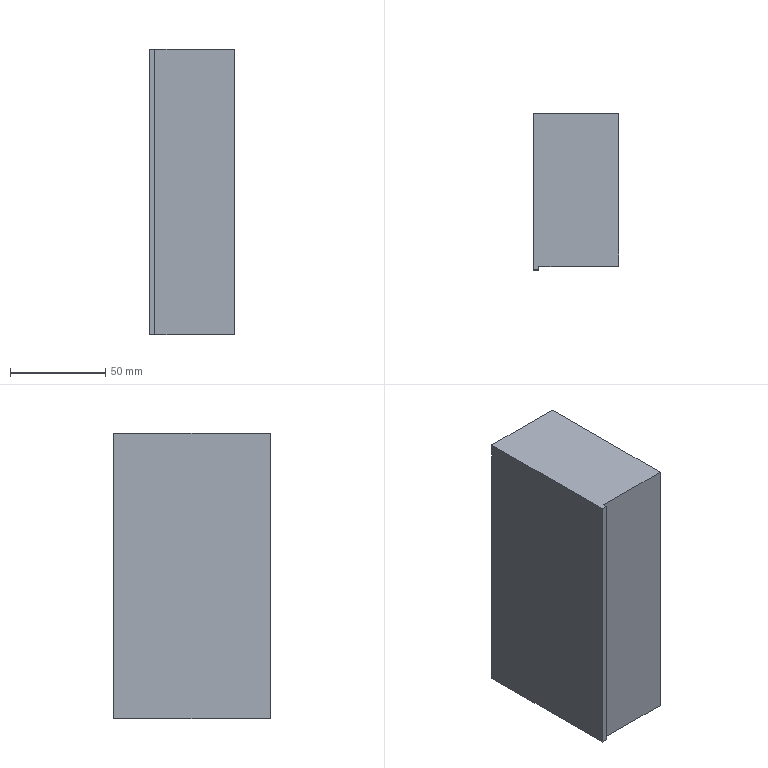Part | SolidWorks | features Extrusion 1 | 1 solid | 8 faces | box 45 x 82 x 150 mm | volume 540900 mm3 | plane 8
STEP:
#1=CARTESIAN_POINT('',(0.,0.,-75.));
#2=VERTEX_POINT('',#1);
#3=CARTESIAN_POINT('',(3.,0.,-75.));
#4=VERTEX_POINT('',#3);
#5=CARTESIAN_POINT('',(3.,0.,-75.));
#6=DIRECTION('',(1.,0.,0.));
#7=VECTOR('',#6,1000.);
#8=LINE('',#5,#7);
#9=EDGE_CURVE('',#2,#4,#8,.T.);
#10=ORIENTED_EDGE('',*,*,#9,.T.);
#11=CARTESIAN_POINT('',(3.,0.,75.));
#12=VERTEX_POINT('',#11);
#13=CARTESIAN_POINT('',(3.,0.,75.));
#14=DIRECTION('',(0.,0.,-1.));
#15=VECTOR('',#14,1000.);
#16=LINE('',#13,#15);
#17=EDGE_CURVE('',#12,#4,#16,.T.);
#18=ORIENTED_EDGE('',*,*,#17,.F.);
#19=CARTESIAN_POINT('',(0.,0.,75.));
#20=VERTEX_POINT('',#19);
#21=CARTESIAN_POINT('',(3.,0.,75.));
#22=DIRECTION('',(1.,0.,0.));
#23=VECTOR('',#22,1000.);
#24=LINE('',#21,#23);
#25=EDGE_CURVE('',#20,#12,#24,.T.);
#26=ORIENTED_EDGE('',*,*,#25,.F.);
#27=CARTESIAN_POINT('',(0.,0.,75.));
#28=DIRECTION('',(0.,0.,-1.));
#29=VECTOR('',#28,1000.);
#30=LINE('',#27,#29);
#31=EDGE_CURVE('',#20,#2,#30,.T.);
#32=ORIENTED_EDGE('',*,*,#31,.T.);
#33=EDGE_LOOP('',(#10,#18,#26,#32));
#34=FACE_OUTER_BOUND('',#33,.T.);
#35=CARTESIAN_POINT('',(3.,0.,75.));
#36=DIRECTION('',(0.,1.,0.));
#37=DIRECTION('',(0.,0.,1.));
#38=AXIS2_PLACEMENT_3D('',#35,#36,#37);
#39=PLANE('',#38);
#40=ADVANCED_FACE('',(#34),#39,.F.);
#41=CARTESIAN_POINT('',(3.,2.,-75.));
#42=VERTEX_POINT('',#41);
#43=CARTESIAN_POINT('',(3.,2.,-75.));
#44=DIRECTION('',(0.,1.,0.));
#45=VECTOR('',#44,1000.);
#46=LINE('',#43,#45);
#47=EDGE_CURVE('',#4,#42,#46,.T.);
#48=ORIENTED_EDGE('',*,*,#47,.T.);
#49=CARTESIAN_POINT('',(3.,2.,75.));
#50=VERTEX_POINT('',#49);
#51=CARTESIAN_POINT('',(3.,2.,75.));
#52=DIRECTION('',(0.,0.,-1.));
#53=VECTOR('',#52,1000.);
#54=LINE('',#51,#53);
#55=EDGE_CURVE('',#50,#42,#54,.T.);
#56=ORIENTED_EDGE('',*,*,#55,.F.);
#57=CARTESIAN_POINT('',(3.,2.,75.));
#58=DIRECTION('',(0.,1.,0.));
#59=VECTOR('',#58,1000.);
#60=LINE('',#57,#59);
#61=EDGE_CURVE('',#12,#50,#60,.T.);
#62=ORIENTED_EDGE('',*,*,#61,.F.);
#63=ORIENTED_EDGE('',*,*,#17,.T.);
#64=EDGE_LOOP('',(#48,#56,#62,#63));
#65=FACE_OUTER_BOUND('',#64,.T.);
#66=CARTESIAN_POINT('',(3.,2.,75.));
#67=DIRECTION('',(-1.,0.,0.));
#68=DIRECTION('',(0.,0.,1.));
#69=AXIS2_PLACEMENT_3D('',#66,#67,#68);
#70=PLANE('',#69);
#71=ADVANCED_FACE('',(#65),#70,.F.);
#72=CARTESIAN_POINT('',(45.,2.,-75.));
#73=VERTEX_POINT('',#72);
#74=CARTESIAN_POINT('',(45.,2.,-75.));
#75=DIRECTION('',(1.,0.,0.));
#76=VECTOR('',#75,1000.);
#77=LINE('',#74,#76);
#78=EDGE_CURVE('',#42,#73,#77,.T.);
#79=ORIENTED_EDGE('',*,*,#78,.T.);
#80=CARTESIAN_POINT('',(45.,2.,75.));
#81=VERTEX_POINT('',#80);
#82=CARTESIAN_POINT('',(45.,2.,75.));
#83=DIRECTION('',(0.,0.,-1.));
#84=VECTOR('',#83,1000.);
#85=LINE('',#82,#84);
#86=EDGE_CURVE('',#81,#73,#85,.T.);
#87=ORIENTED_EDGE('',*,*,#86,.F.);
#88=CARTESIAN_POINT('',(45.,2.,75.));
#89=DIRECTION('',(1.,0.,0.));
#90=VECTOR('',#89,1000.);
#91=LINE('',#88,#90);
#92=EDGE_CURVE('',#50,#81,#91,.T.);
#93=ORIENTED_EDGE('',*,*,#92,.F.);
#94=ORIENTED_EDGE('',*,*,#55,.T.);
#95=EDGE_LOOP('',(#79,#87,#93,#94));
#96=FACE_OUTER_BOUND('',#95,.T.);
#97=CARTESIAN_POINT('',(45.,2.,75.));
#98=DIRECTION('',(0.,1.,0.));
#99=DIRECTION('',(-1.,0.,0.));
#100=AXIS2_PLACEMENT_3D('',#97,#98,#99);
#101=PLANE('',#100);
#102=ADVANCED_FACE('',(#96),#101,.F.);
#103=CARTESIAN_POINT('',(45.,82.,-75.));
#104=VERTEX_POINT('',#103);
#105=CARTESIAN_POINT('',(45.,82.,-75.));
#106=DIRECTION('',(0.,1.,0.));
#107=VECTOR('',#106,1000.);
#108=LINE('',#105,#107);
#109=EDGE_CURVE('',#73,#104,#108,.T.);
#110=ORIENTED_EDGE('',*,*,#109,.T.);
#111=CARTESIAN_POINT('',(45.,82.,75.));
#112=VERTEX_POINT('',#111);
#113=CARTESIAN_POINT('',(45.,82.,75.));
#114=DIRECTION('',(0.,0.,-1.));
#115=VECTOR('',#114,1000.);
#116=LINE('',#113,#115);
#117=EDGE_CURVE('',#112,#104,#116,.T.);
#118=ORIENTED_EDGE('',*,*,#117,.F.);
#119=CARTESIAN_POINT('',(45.,82.,75.));
#120=DIRECTION('',(0.,1.,0.));
#121=VECTOR('',#120,1000.);
#122=LINE('',#119,#121);
#123=EDGE_CURVE('',#81,#112,#122,.T.);
#124=ORIENTED_EDGE('',*,*,#123,.F.);
#125=ORIENTED_EDGE('',*,*,#86,.T.);
#126=EDGE_LOOP('',(#110,#118,#124,#125));
#127=FACE_OUTER_BOUND('',#126,.T.);
#128=CARTESIAN_POINT('',(45.,82.,75.));
#129=DIRECTION('',(-1.,0.,0.));
#130=DIRECTION('',(0.,-1.,0.));
#131=AXIS2_PLACEMENT_3D('',#128,#129,#130);
#132=PLANE('',#131);
#133=ADVANCED_FACE('',(#127),#132,.F.);
#134=CARTESIAN_POINT('',(0.,82.,-75.));
#135=VERTEX_POINT('',#134);
#136=CARTESIAN_POINT('',(0.,82.,-75.));
#137=DIRECTION('',(-1.,0.,0.));
#138=VECTOR('',#137,1000.);
#139=LINE('',#136,#138);
#140=EDGE_CURVE('',#104,#135,#139,.T.);
#141=ORIENTED_EDGE('',*,*,#140,.T.);
#142=CARTESIAN_POINT('',(0.,82.,75.));
#143=VERTEX_POINT('',#142);
#144=CARTESIAN_POINT('',(0.,82.,75.));
#145=DIRECTION('',(0.,0.,-1.));
#146=VECTOR('',#145,1000.);
#147=LINE('',#144,#146);
#148=EDGE_CURVE('',#143,#135,#147,.T.);
#149=ORIENTED_EDGE('',*,*,#148,.F.);
#150=CARTESIAN_POINT('',(0.,82.,75.));
#151=DIRECTION('',(-1.,0.,0.));
#152=VECTOR('',#151,1000.);
#153=LINE('',#150,#152);
#154=EDGE_CURVE('',#112,#143,#153,.T.);
#155=ORIENTED_EDGE('',*,*,#154,.F.);
#156=ORIENTED_EDGE('',*,*,#117,.T.);
#157=EDGE_LOOP('',(#141,#149,#155,#156));
#158=FACE_OUTER_BOUND('',#157,.T.);
#159=CARTESIAN_POINT('',(0.,82.,75.));
#160=DIRECTION('',(0.,-1.,0.));
#161=DIRECTION('',(0.,0.,-1.));
#162=AXIS2_PLACEMENT_3D('',#159,#160,#161);
#163=PLANE('',#162);
#164=ADVANCED_FACE('',(#158),#163,.F.);
#165=CARTESIAN_POINT('',(0.,0.,-75.));
#166=DIRECTION('',(0.,-1.,0.));
#167=VECTOR('',#166,1000.);
#168=LINE('',#165,#167);
#169=EDGE_CURVE('',#135,#2,#168,.T.);
#170=ORIENTED_EDGE('',*,*,#169,.T.);
#171=ORIENTED_EDGE('',*,*,#31,.F.);
#172=CARTESIAN_POINT('',(0.,0.,75.));
#173=DIRECTION('',(0.,-1.,0.));
#174=VECTOR('',#173,1000.);
#175=LINE('',#172,#174);
#176=EDGE_CURVE('',#143,#20,#175,.T.);
#177=ORIENTED_EDGE('',*,*,#176,.F.);
#178=ORIENTED_EDGE('',*,*,#148,.T.);
#179=EDGE_LOOP('',(#170,#171,#177,#178));
#180=FACE_OUTER_BOUND('',#179,.T.);
#181=CARTESIAN_POINT('',(0.,0.,75.));
#182=DIRECTION('',(1.,0.,0.));
#183=DIRECTION('',(0.,0.,-1.));
#184=AXIS2_PLACEMENT_3D('',#181,#182,#183);
#185=PLANE('',#184);
#186=ADVANCED_FACE('',(#180),#185,.F.);
#187=ORIENTED_EDGE('',*,*,#25,.T.);
#188=ORIENTED_EDGE('',*,*,#61,.T.);
#189=ORIENTED_EDGE('',*,*,#92,.T.);
#190=ORIENTED_EDGE('',*,*,#123,.T.);
#191=ORIENTED_EDGE('',*,*,#154,.T.);
#192=ORIENTED_EDGE('',*,*,#176,.T.);
#193=EDGE_LOOP('',(#187,#188,#189,#190,#191,#192));
#194=FACE_OUTER_BOUND('',#193,.T.);
#195=CARTESIAN_POINT('',(0.,0.,75.));
#196=DIRECTION('',(0.,0.,-1.));
#197=DIRECTION('',(-1.,0.,0.));
#198=AXIS2_PLACEMENT_3D('',#195,#196,#197);
#199=PLANE('',#198);
#200=ADVANCED_FACE('',(#194),#199,.F.);
#201=ORIENTED_EDGE('',*,*,#9,.F.);
#202=ORIENTED_EDGE('',*,*,#169,.F.);
#203=ORIENTED_EDGE('',*,*,#140,.F.);
#204=ORIENTED_EDGE('',*,*,#109,.F.);
#205=ORIENTED_EDGE('',*,*,#78,.F.);
#206=ORIENTED_EDGE('',*,*,#47,.F.);
#207=EDGE_LOOP('',(#201,#202,#203,#204,#205,#206));
#208=FACE_OUTER_BOUND('',#207,.T.);
#209=CARTESIAN_POINT('',(0.,0.,-75.));
#210=DIRECTION('',(0.,0.,-1.));
#211=DIRECTION('',(-1.,0.,0.));
#212=AXIS2_PLACEMENT_3D('',#209,#210,#211);
#213=PLANE('',#212);
#214=ADVANCED_FACE('',(#208),#213,.T.);
#215=CLOSED_SHELL('',(#40,#71,#102,#133,#164,#186,#200,#214));
#216=MANIFOLD_SOLID_BREP('',#215);
#217=CARTESIAN_POINT('',(0.,0.,0.));
#218=DIRECTION('',(0.,0.,1.));
#219=DIRECTION('',(1.,0.,0.));
#220=AXIS2_PLACEMENT_3D('',#217,#218,#219);
#221=(LENGTH_UNIT()NAMED_UNIT(*)SI_UNIT(.MILLI.,.METRE.));
#222=UNCERTAINTY_MEASURE_WITH_UNIT(LENGTH_MEASURE(0.00001),#221,'','');
#223=(NAMED_UNIT(*)PLANE_ANGLE_UNIT()SI_UNIT($,.RADIAN.));
#224=(NAMED_UNIT(*)SI_UNIT($,.STERADIAN.)SOLID_ANGLE_UNIT());
#225=(GEOMETRIC_REPRESENTATION_CONTEXT(3)GLOBAL_UNCERTAINTY_ASSIGNED_CONTEXT((#222))GLOBAL_UNIT_ASSIGNED_CONTEXT((#221,#223,#224))REPRESENTATION_CONTEXT('',''));
#226=ADVANCED_BREP_SHAPE_REPRESENTATION('',(#216,#220),#225);